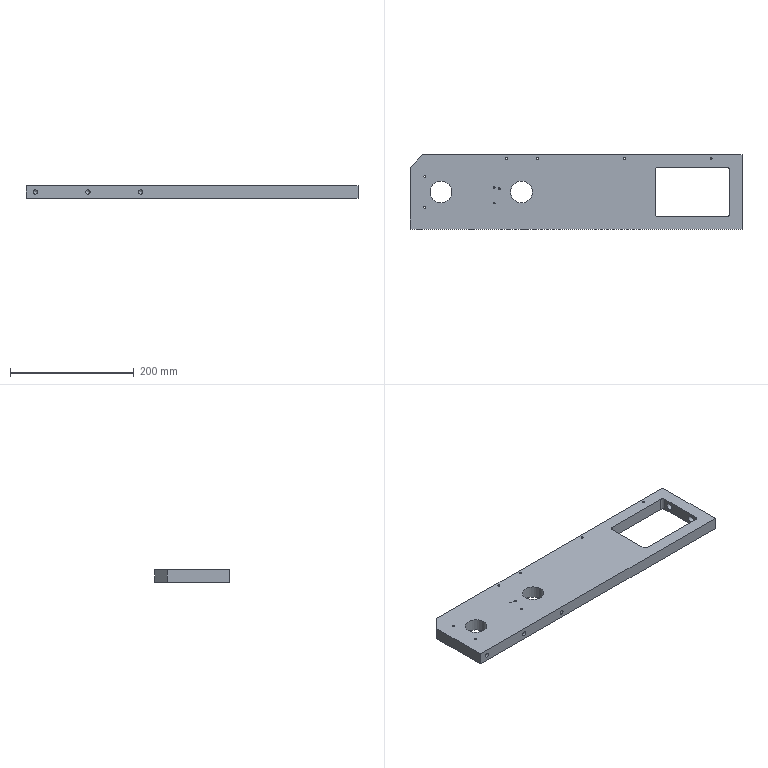Part | NX | 1 solid | 36 faces | box 536 x 120 x 20 mm | volume 1044762 mm3 | cylinder 20 | plane 11 | cone 5 | commonest cylinder face diameters 3.3 x7 10 x4 6.8 x3 2.5 x2 11 x2 35 x2
STEP:
#1=CARTESIAN_POINT('',(-248.,60.,10.));
#2=VERTEX_POINT('',#1);
#3=CARTESIAN_POINT('',(-268.,40.,10.));
#4=VERTEX_POINT('',#3);
#5=CARTESIAN_POINT('',(-268.,40.,10.));
#6=DIRECTION('',(-0.7071,-0.7071,0.));
#7=VECTOR('',#6,1000.);
#8=LINE('',#5,#7);
#9=EDGE_CURVE('',#2,#4,#8,.T.);
#10=ORIENTED_EDGE('',*,*,#9,.F.);
#11=CARTESIAN_POINT('',(-248.,60.,-10.));
#12=VERTEX_POINT('',#11);
#13=CARTESIAN_POINT('',(-248.,60.,10.));
#14=DIRECTION('',(0.,0.,1.));
#15=VECTOR('',#14,1000.);
#16=LINE('',#13,#15);
#17=EDGE_CURVE('',#12,#2,#16,.T.);
#18=ORIENTED_EDGE('',*,*,#17,.F.);
#19=CARTESIAN_POINT('',(-268.,40.,-10.));
#20=VERTEX_POINT('',#19);
#21=CARTESIAN_POINT('',(-154.,154.,-10.));
#22=DIRECTION('',(0.7071,0.7071,0.));
#23=VECTOR('',#22,1000.);
#24=LINE('',#21,#23);
#25=EDGE_CURVE('',#20,#12,#24,.T.);
#26=ORIENTED_EDGE('',*,*,#25,.F.);
#27=CARTESIAN_POINT('',(-268.,40.,10.));
#28=DIRECTION('',(0.,0.,-1.));
#29=VECTOR('',#28,1000.);
#30=LINE('',#27,#29);
#31=EDGE_CURVE('',#4,#20,#30,.T.);
#32=ORIENTED_EDGE('',*,*,#31,.F.);
#33=EDGE_LOOP('',(#10,#18,#26,#32));
#34=FACE_BOUND('',#33,.T.);
#35=CARTESIAN_POINT('',(-268.,40.,10.));
#36=DIRECTION('',(0.7071,-0.7071,0.));
#37=DIRECTION('',(0.,0.,-1.));
#38=AXIS2_PLACEMENT_3D('',#35,#36,#37);
#39=PLANE('',#38);
#40=ADVANCED_FACE('',(#34),#39,.F.);
#41=CARTESIAN_POINT('',(248.,-35.,10.));
#42=VERTEX_POINT('',#41);
#43=CARTESIAN_POINT('',(248.,35.,10.));
#44=VERTEX_POINT('',#43);
#45=CARTESIAN_POINT('',(248.,-35.,10.));
#46=DIRECTION('',(0.,1.,0.));
#47=VECTOR('',#46,1000.);
#48=LINE('',#45,#47);
#49=EDGE_CURVE('',#42,#44,#48,.T.);
#50=ORIENTED_EDGE('',*,*,#49,.T.);
#51=CARTESIAN_POINT('',(248.,35.,-10.));
#52=VERTEX_POINT('',#51);
#53=CARTESIAN_POINT('',(248.,35.,-10.));
#54=DIRECTION('',(0.,0.,1.));
#55=VECTOR('',#54,1000.);
#56=LINE('',#53,#55);
#57=EDGE_CURVE('',#52,#44,#56,.T.);
#58=ORIENTED_EDGE('',*,*,#57,.F.);
#59=CARTESIAN_POINT('',(248.,-35.,-10.));
#60=VERTEX_POINT('',#59);
#61=CARTESIAN_POINT('',(248.,-35.,-10.));
#62=DIRECTION('',(0.,1.,0.));
#63=VECTOR('',#62,1000.);
#64=LINE('',#61,#63);
#65=EDGE_CURVE('',#60,#52,#64,.T.);
#66=ORIENTED_EDGE('',*,*,#65,.F.);
#67=CARTESIAN_POINT('',(248.,-35.,-10.));
#68=DIRECTION('',(0.,0.,1.));
#69=VECTOR('',#68,1000.);
#70=LINE('',#67,#69);
#71=EDGE_CURVE('',#60,#42,#70,.T.);
#72=ORIENTED_EDGE('',*,*,#71,.T.);
#73=EDGE_LOOP('',(#50,#58,#66,#72));
#74=FACE_BOUND('',#73,.T.);
#75=CARTESIAN_POINT('',(248.,25.,-5.5));
#76=VERTEX_POINT('',#75);
#77=CARTESIAN_POINT('',(248.,25.,0.));
#78=DIRECTION('',(1.,0.,0.));
#79=DIRECTION('',(0.,0.,-1.));
#80=AXIS2_PLACEMENT_3D('',#77,#78,#79);
#81=CIRCLE('',#80,5.5);
#82=EDGE_CURVE('',#76,#76,#81,.T.);
#83=ORIENTED_EDGE('',*,*,#82,.T.);
#84=EDGE_LOOP('',(#83));
#85=FACE_BOUND('',#84,.T.);
#86=CARTESIAN_POINT('',(248.,-25.,-5.5));
#87=VERTEX_POINT('',#86);
#88=CARTESIAN_POINT('',(248.,-25.,0.));
#89=DIRECTION('',(1.,0.,0.));
#90=DIRECTION('',(0.,0.,-1.));
#91=AXIS2_PLACEMENT_3D('',#88,#89,#90);
#92=CIRCLE('',#91,5.5);
#93=EDGE_CURVE('',#87,#87,#92,.T.);
#94=ORIENTED_EDGE('',*,*,#93,.T.);
#95=EDGE_LOOP('',(#94));
#96=FACE_BOUND('',#95,.T.);
#97=CARTESIAN_POINT('',(248.,-35.,-10.));
#98=DIRECTION('',(1.,0.,0.));
#99=DIRECTION('',(0.,0.,-1.));
#100=AXIS2_PLACEMENT_3D('',#97,#98,#99);
#101=PLANE('',#100);
#102=ADVANCED_FACE('',(#74,#85,#96),#101,.F.);
#103=CARTESIAN_POINT('',(243.,40.,10.));
#104=VERTEX_POINT('',#103);
#105=CARTESIAN_POINT('',(243.,35.,10.));
#106=DIRECTION('',(0.,0.,1.));
#107=DIRECTION('',(-1.,0.,0.));
#108=AXIS2_PLACEMENT_3D('',#105,#106,#107);
#109=CIRCLE('',#108,5.);
#110=EDGE_CURVE('',#44,#104,#109,.T.);
#111=ORIENTED_EDGE('',*,*,#110,.T.);
#112=CARTESIAN_POINT('',(243.,40.,-10.));
#113=VERTEX_POINT('',#112);
#114=CARTESIAN_POINT('',(243.,40.,-10.));
#115=DIRECTION('',(0.,0.,1.));
#116=VECTOR('',#115,1000.);
#117=LINE('',#114,#116);
#118=EDGE_CURVE('',#113,#104,#117,.T.);
#119=ORIENTED_EDGE('',*,*,#118,.F.);
#120=CARTESIAN_POINT('',(243.,35.,-10.));
#121=DIRECTION('',(0.,0.,1.));
#122=DIRECTION('',(-1.,0.,0.));
#123=AXIS2_PLACEMENT_3D('',#120,#121,#122);
#124=CIRCLE('',#123,5.);
#125=EDGE_CURVE('',#52,#113,#124,.T.);
#126=ORIENTED_EDGE('',*,*,#125,.F.);
#127=ORIENTED_EDGE('',*,*,#57,.T.);
#128=EDGE_LOOP('',(#111,#119,#126,#127));
#129=FACE_BOUND('',#128,.T.);
#130=CARTESIAN_POINT('',(243.,35.,-10.));
#131=DIRECTION('',(0.,0.,1.));
#132=DIRECTION('',(1.,0.,0.));
#133=AXIS2_PLACEMENT_3D('',#130,#131,#132);
#134=CYLINDRICAL_SURFACE('',#133,5.);
#135=ADVANCED_FACE('',(#129),#134,.F.);
#136=CARTESIAN_POINT('',(133.,40.,10.));
#137=VERTEX_POINT('',#136);
#138=CARTESIAN_POINT('',(133.,40.,10.));
#139=DIRECTION('',(-1.,0.,0.));
#140=VECTOR('',#139,1000.);
#141=LINE('',#138,#140);
#142=EDGE_CURVE('',#104,#137,#141,.T.);
#143=ORIENTED_EDGE('',*,*,#142,.T.);
#144=CARTESIAN_POINT('',(133.,40.,-10.));
#145=VERTEX_POINT('',#144);
#146=CARTESIAN_POINT('',(133.,40.,-10.));
#147=DIRECTION('',(0.,0.,1.));
#148=VECTOR('',#147,1000.);
#149=LINE('',#146,#148);
#150=EDGE_CURVE('',#145,#137,#149,.T.);
#151=ORIENTED_EDGE('',*,*,#150,.F.);
#152=CARTESIAN_POINT('',(133.,40.,-10.));
#153=DIRECTION('',(-1.,0.,0.));
#154=VECTOR('',#153,1000.);
#155=LINE('',#152,#154);
#156=EDGE_CURVE('',#113,#145,#155,.T.);
#157=ORIENTED_EDGE('',*,*,#156,.F.);
#158=ORIENTED_EDGE('',*,*,#118,.T.);
#159=EDGE_LOOP('',(#143,#151,#157,#158));
#160=FACE_BOUND('',#159,.T.);
#161=CARTESIAN_POINT('',(133.,40.,-10.));
#162=DIRECTION('',(0.,1.,0.));
#163=DIRECTION('',(-1.,0.,0.));
#164=AXIS2_PLACEMENT_3D('',#161,#162,#163);
#165=PLANE('',#164);
#166=ADVANCED_FACE('',(#160),#165,.F.);
#167=CARTESIAN_POINT('',(128.,35.,10.));
#168=VERTEX_POINT('',#167);
#169=CARTESIAN_POINT('',(133.,35.,10.));
#170=DIRECTION('',(0.,0.,1.));
#171=DIRECTION('',(-1.,0.,0.));
#172=AXIS2_PLACEMENT_3D('',#169,#170,#171);
#173=CIRCLE('',#172,5.);
#174=EDGE_CURVE('',#137,#168,#173,.T.);
#175=ORIENTED_EDGE('',*,*,#174,.T.);
#176=CARTESIAN_POINT('',(128.,35.,-10.));
#177=VERTEX_POINT('',#176);
#178=CARTESIAN_POINT('',(128.,35.,-10.));
#179=DIRECTION('',(0.,0.,1.));
#180=VECTOR('',#179,1000.);
#181=LINE('',#178,#180);
#182=EDGE_CURVE('',#177,#168,#181,.T.);
#183=ORIENTED_EDGE('',*,*,#182,.F.);
#184=CARTESIAN_POINT('',(133.,35.,-10.));
#185=DIRECTION('',(0.,0.,1.));
#186=DIRECTION('',(-1.,0.,0.));
#187=AXIS2_PLACEMENT_3D('',#184,#185,#186);
#188=CIRCLE('',#187,5.);
#189=EDGE_CURVE('',#145,#177,#188,.T.);
#190=ORIENTED_EDGE('',*,*,#189,.F.);
#191=ORIENTED_EDGE('',*,*,#150,.T.);
#192=EDGE_LOOP('',(#175,#183,#190,#191));
#193=FACE_BOUND('',#192,.T.);
#194=CARTESIAN_POINT('',(133.,35.,-10.));
#195=DIRECTION('',(0.,0.,1.));
#196=DIRECTION('',(1.,0.,0.));
#197=AXIS2_PLACEMENT_3D('',#194,#195,#196);
#198=CYLINDRICAL_SURFACE('',#197,5.);
#199=ADVANCED_FACE('',(#193),#198,.F.);
#200=CARTESIAN_POINT('',(128.,-35.,10.));
#201=VERTEX_POINT('',#200);
#202=CARTESIAN_POINT('',(128.,-35.,10.));
#203=DIRECTION('',(0.,-1.,0.));
#204=VECTOR('',#203,1000.);
#205=LINE('',#202,#204);
#206=EDGE_CURVE('',#168,#201,#205,.T.);
#207=ORIENTED_EDGE('',*,*,#206,.T.);
#208=CARTESIAN_POINT('',(128.,-35.,-10.));
#209=VERTEX_POINT('',#208);
#210=CARTESIAN_POINT('',(128.,-35.,-10.));
#211=DIRECTION('',(0.,0.,1.));
#212=VECTOR('',#211,1000.);
#213=LINE('',#210,#212);
#214=EDGE_CURVE('',#209,#201,#213,.T.);
#215=ORIENTED_EDGE('',*,*,#214,.F.);
#216=CARTESIAN_POINT('',(128.,-35.,-10.));
#217=DIRECTION('',(0.,-1.,0.));
#218=VECTOR('',#217,1000.);
#219=LINE('',#216,#218);
#220=EDGE_CURVE('',#177,#209,#219,.T.);
#221=ORIENTED_EDGE('',*,*,#220,.F.);
#222=ORIENTED_EDGE('',*,*,#182,.T.);
#223=EDGE_LOOP('',(#207,#215,#221,#222));
#224=FACE_BOUND('',#223,.T.);
#225=CARTESIAN_POINT('',(128.,-35.,-10.));
#226=DIRECTION('',(-1.,0.,0.));
#227=DIRECTION('',(0.,0.,1.));
#228=AXIS2_PLACEMENT_3D('',#225,#226,#227);
#229=PLANE('',#228);
#230=ADVANCED_FACE('',(#224),#229,.F.);
#231=CARTESIAN_POINT('',(133.,-40.,10.));
#232=VERTEX_POINT('',#231);
#233=CARTESIAN_POINT('',(133.,-35.,10.));
#234=DIRECTION('',(0.,0.,1.));
#235=DIRECTION('',(-1.,0.,0.));
#236=AXIS2_PLACEMENT_3D('',#233,#234,#235);
#237=CIRCLE('',#236,5.);
#238=EDGE_CURVE('',#201,#232,#237,.T.);
#239=ORIENTED_EDGE('',*,*,#238,.T.);
#240=CARTESIAN_POINT('',(133.,-40.,-10.));
#241=VERTEX_POINT('',#240);
#242=CARTESIAN_POINT('',(133.,-40.,-10.));
#243=DIRECTION('',(0.,0.,1.));
#244=VECTOR('',#243,1000.);
#245=LINE('',#242,#244);
#246=EDGE_CURVE('',#241,#232,#245,.T.);
#247=ORIENTED_EDGE('',*,*,#246,.F.);
#248=CARTESIAN_POINT('',(133.,-35.,-10.));
#249=DIRECTION('',(0.,0.,1.));
#250=DIRECTION('',(-1.,0.,0.));
#251=AXIS2_PLACEMENT_3D('',#248,#249,#250);
#252=CIRCLE('',#251,5.);
#253=EDGE_CURVE('',#209,#241,#252,.T.);
#254=ORIENTED_EDGE('',*,*,#253,.F.);
#255=ORIENTED_EDGE('',*,*,#214,.T.);
#256=EDGE_LOOP('',(#239,#247,#254,#255));
#257=FACE_BOUND('',#256,.T.);
#258=CARTESIAN_POINT('',(133.,-35.,-10.));
#259=DIRECTION('',(0.,0.,1.));
#260=DIRECTION('',(1.,0.,0.));
#261=AXIS2_PLACEMENT_3D('',#258,#259,#260);
#262=CYLINDRICAL_SURFACE('',#261,5.);
#263=ADVANCED_FACE('',(#257),#262,.F.);
#264=CARTESIAN_POINT('',(243.,-40.,10.));
#265=VERTEX_POINT('',#264);
#266=CARTESIAN_POINT('',(133.,-40.,10.));
#267=DIRECTION('',(1.,0.,0.));
#268=VECTOR('',#267,1000.);
#269=LINE('',#266,#268);
#270=EDGE_CURVE('',#232,#265,#269,.T.);
#271=ORIENTED_EDGE('',*,*,#270,.T.);
#272=CARTESIAN_POINT('',(243.,-40.,-10.));
#273=VERTEX_POINT('',#272);
#274=CARTESIAN_POINT('',(243.,-40.,-10.));
#275=DIRECTION('',(0.,0.,1.));
#276=VECTOR('',#275,1000.);
#277=LINE('',#274,#276);
#278=EDGE_CURVE('',#273,#265,#277,.T.);
#279=ORIENTED_EDGE('',*,*,#278,.F.);
#280=CARTESIAN_POINT('',(133.,-40.,-10.));
#281=DIRECTION('',(1.,0.,0.));
#282=VECTOR('',#281,1000.);
#283=LINE('',#280,#282);
#284=EDGE_CURVE('',#241,#273,#283,.T.);
#285=ORIENTED_EDGE('',*,*,#284,.F.);
#286=ORIENTED_EDGE('',*,*,#246,.T.);
#287=EDGE_LOOP('',(#271,#279,#285,#286));
#288=FACE_BOUND('',#287,.T.);
#289=CARTESIAN_POINT('',(133.,-40.,-10.));
#290=DIRECTION('',(0.,-1.,0.));
#291=DIRECTION('',(0.,0.,-1.));
#292=AXIS2_PLACEMENT_3D('',#289,#290,#291);
#293=PLANE('',#292);
#294=ADVANCED_FACE('',(#288),#293,.F.);
#295=CARTESIAN_POINT('',(243.,-35.,10.));
#296=DIRECTION('',(0.,0.,1.));
#297=DIRECTION('',(1.,0.,0.));
#298=AXIS2_PLACEMENT_3D('',#295,#296,#297);
#299=CIRCLE('',#298,5.);
#300=EDGE_CURVE('',#265,#42,#299,.T.);
#301=ORIENTED_EDGE('',*,*,#300,.T.);
#302=ORIENTED_EDGE('',*,*,#71,.F.);
#303=CARTESIAN_POINT('',(243.,-35.,-10.));
#304=DIRECTION('',(0.,0.,1.));
#305=DIRECTION('',(1.,0.,0.));
#306=AXIS2_PLACEMENT_3D('',#303,#304,#305);
#307=CIRCLE('',#306,5.);
#308=EDGE_CURVE('',#273,#60,#307,.T.);
#309=ORIENTED_EDGE('',*,*,#308,.F.);
#310=ORIENTED_EDGE('',*,*,#278,.T.);
#311=EDGE_LOOP('',(#301,#302,#309,#310));
#312=FACE_BOUND('',#311,.T.);
#313=CARTESIAN_POINT('',(243.,-35.,-10.));
#314=DIRECTION('',(0.,0.,1.));
#315=DIRECTION('',(1.,0.,0.));
#316=AXIS2_PLACEMENT_3D('',#313,#314,#315);
#317=CYLINDRICAL_SURFACE('',#316,5.);
#318=ADVANCED_FACE('',(#312),#317,.F.);
#319=ORIENTED_EDGE('',*,*,#308,.T.);
#320=ORIENTED_EDGE('',*,*,#65,.T.);
#321=ORIENTED_EDGE('',*,*,#125,.T.);
#322=ORIENTED_EDGE('',*,*,#156,.T.);
#323=ORIENTED_EDGE('',*,*,#189,.T.);
#324=ORIENTED_EDGE('',*,*,#220,.T.);
#325=ORIENTED_EDGE('',*,*,#253,.T.);
#326=ORIENTED_EDGE('',*,*,#284,.T.);
#327=EDGE_LOOP('',(#319,#320,#321,#322,#323,#324,#325,#326));
#328=FACE_BOUND('',#327,.T.);
#329=CARTESIAN_POINT('',(-268.,-60.,-10.));
#330=VERTEX_POINT('',#329);
#331=CARTESIAN_POINT('',(-268.,-60.,-10.));
#332=DIRECTION('',(0.,-1.,0.));
#333=VECTOR('',#332,1000.);
#334=LINE('',#331,#333);
#335=EDGE_CURVE('',#20,#330,#334,.T.);
#336=ORIENTED_EDGE('',*,*,#335,.F.);
#337=ORIENTED_EDGE('',*,*,#25,.T.);
#338=CARTESIAN_POINT('',(268.,60.,-10.));
#339=VERTEX_POINT('',#338);
#340=CARTESIAN_POINT('',(-268.,60.,-10.));
#341=DIRECTION('',(-1.,0.,0.));
#342=VECTOR('',#341,1000.);
#343=LINE('',#340,#342);
#344=EDGE_CURVE('',#339,#12,#343,.T.);
#345=ORIENTED_EDGE('',*,*,#344,.F.);
#346=CARTESIAN_POINT('',(268.,-60.,-10.));
#347=VERTEX_POINT('',#346);
#348=CARTESIAN_POINT('',(268.,-60.,-10.));
#349=DIRECTION('',(0.,1.,0.));
#350=VECTOR('',#349,1000.);
#351=LINE('',#348,#350);
#352=EDGE_CURVE('',#339,#347,#351,.F.);
#353=ORIENTED_EDGE('',*,*,#352,.T.);
#354=CARTESIAN_POINT('',(-268.,-60.,-10.));
#355=DIRECTION('',(1.,0.,0.));
#356=VECTOR('',#355,1000.);
#357=LINE('',#354,#356);
#358=EDGE_CURVE('',#330,#347,#357,.T.);
#359=ORIENTED_EDGE('',*,*,#358,.F.);
#360=EDGE_LOOP('',(#336,#337,#345,#353,#359));
#361=FACE_BOUND('',#360,.T.);
#362=CARTESIAN_POINT('',(-245.65,25.,-10.));
#363=VERTEX_POINT('',#362);
#364=CARTESIAN_POINT('',(-244.,25.,-10.));
#365=DIRECTION('',(0.,0.,-1.));
#366=DIRECTION('',(-1.,0.,0.));
#367=AXIS2_PLACEMENT_3D('',#364,#365,#366);
#368=CIRCLE('',#367,1.65);
#369=EDGE_CURVE('',#363,#363,#368,.T.);
#370=ORIENTED_EDGE('',*,*,#369,.F.);
#371=EDGE_LOOP('',(#370));
#372=FACE_BOUND('',#371,.T.);
#373=CARTESIAN_POINT('',(-245.65,-25.,-10.));
#374=VERTEX_POINT('',#373);
#375=CARTESIAN_POINT('',(-244.,-25.,-10.));
#376=DIRECTION('',(0.,0.,-1.));
#377=DIRECTION('',(-1.,0.,0.));
#378=AXIS2_PLACEMENT_3D('',#375,#376,#377);
#379=CIRCLE('',#378,1.65);
#380=EDGE_CURVE('',#374,#374,#379,.T.);
#381=ORIENTED_EDGE('',*,*,#380,.F.);
#382=EDGE_LOOP('',(#381));
#383=FACE_BOUND('',#382,.T.);
#384=CARTESIAN_POINT('',(-70.5,0.,-10.));
#385=VERTEX_POINT('',#384);
#386=CARTESIAN_POINT('',(-88.,0.,-10.));
#387=DIRECTION('',(0.,0.,1.));
#388=DIRECTION('',(1.,0.,0.));
#389=AXIS2_PLACEMENT_3D('',#386,#387,#388);
#390=CIRCLE('',#389,17.5);
#391=EDGE_CURVE('',#385,#385,#390,.T.);
#392=ORIENTED_EDGE('',*,*,#391,.T.);
#393=EDGE_LOOP('',(#392));
#394=FACE_BOUND('',#393,.T.);
#395=CARTESIAN_POINT('',(-200.5,0.,-10.));
#396=VERTEX_POINT('',#395);
#397=CARTESIAN_POINT('',(-218.,0.,-10.));
#398=DIRECTION('',(0.,0.,1.));
#399=DIRECTION('',(1.,0.,0.));
#400=AXIS2_PLACEMENT_3D('',#397,#398,#399);
#401=CIRCLE('',#400,17.5);
#402=EDGE_CURVE('',#396,#396,#401,.T.);
#403=ORIENTED_EDGE('',*,*,#402,.T.);
#404=EDGE_LOOP('',(#403));
#405=FACE_BOUND('',#404,.T.);
#406=CARTESIAN_POINT('',(219.65,54.25,-10.));
#407=VERTEX_POINT('',#406);
#408=CARTESIAN_POINT('',(218.,54.25,-10.));
#409=DIRECTION('',(0.,0.,1.));
#410=DIRECTION('',(1.,0.,0.));
#411=AXIS2_PLACEMENT_3D('',#408,#409,#410);
#412=CIRCLE('',#411,1.65);
#413=EDGE_CURVE('',#407,#407,#412,.T.);
#414=ORIENTED_EDGE('',*,*,#413,.T.);
#415=EDGE_LOOP('',(#414));
#416=FACE_BOUND('',#415,.T.);
#417=CARTESIAN_POINT('',(79.65,54.25,-10.));
#418=VERTEX_POINT('',#417);
#419=CARTESIAN_POINT('',(78.,54.25,-10.));
#420=DIRECTION('',(0.,0.,1.));
#421=DIRECTION('',(1.,0.,0.));
#422=AXIS2_PLACEMENT_3D('',#419,#420,#421);
#423=CIRCLE('',#422,1.65);
#424=EDGE_CURVE('',#418,#418,#423,.T.);
#425=ORIENTED_EDGE('',*,*,#424,.T.);
#426=EDGE_LOOP('',(#425));
#427=FACE_BOUND('',#426,.T.);
#428=CARTESIAN_POINT('',(-60.35,54.25,-10.));
#429=VERTEX_POINT('',#428);
#430=CARTESIAN_POINT('',(-62.,54.25,-10.));
#431=DIRECTION('',(0.,0.,1.));
#432=DIRECTION('',(1.,0.,0.));
#433=AXIS2_PLACEMENT_3D('',#430,#431,#432);
#434=CIRCLE('',#433,1.65);
#435=EDGE_CURVE('',#429,#429,#434,.T.);
#436=ORIENTED_EDGE('',*,*,#435,.T.);
#437=EDGE_LOOP('',(#436));
#438=FACE_BOUND('',#437,.T.);
#439=CARTESIAN_POINT('',(-110.35,54.25,-10.));
#440=VERTEX_POINT('',#439);
#441=CARTESIAN_POINT('',(-112.,54.25,-10.));
#442=DIRECTION('',(0.,0.,1.));
#443=DIRECTION('',(1.,0.,0.));
#444=AXIS2_PLACEMENT_3D('',#441,#442,#443);
#445=CIRCLE('',#444,1.65);
#446=EDGE_CURVE('',#440,#440,#445,.T.);
#447=ORIENTED_EDGE('',*,*,#446,.T.);
#448=EDGE_LOOP('',(#447));
#449=FACE_BOUND('',#448,.T.);
#450=CARTESIAN_POINT('',(-122.35,5.25,-10.));
#451=VERTEX_POINT('',#450);
#452=CARTESIAN_POINT('',(-124.,5.25,-10.));
#453=DIRECTION('',(0.,0.,1.));
#454=DIRECTION('',(1.,0.,0.));
#455=AXIS2_PLACEMENT_3D('',#452,#453,#454);
#456=CIRCLE('',#455,1.65);
#457=EDGE_CURVE('',#451,#451,#456,.T.);
#458=ORIENTED_EDGE('',*,*,#457,.T.);
#459=EDGE_LOOP('',(#458));
#460=FACE_BOUND('',#459,.T.);
#461=CARTESIAN_POINT('',(0.,0.,-10.));
#462=DIRECTION('',(0.,0.,-1.));
#463=DIRECTION('',(-1.,0.,0.));
#464=AXIS2_PLACEMENT_3D('',#461,#462,#463);
#465=PLANE('',#464);
#466=ADVANCED_FACE('',(#328,#361,#372,#383,#394,#405,#416,#427,#438,#449,#460),#465,.T.);
#467=CARTESIAN_POINT('',(268.,60.,10.));
#468=VERTEX_POINT('',#467);
#469=CARTESIAN_POINT('',(-268.,60.,10.));
#470=DIRECTION('',(-1.,0.,0.));
#471=VECTOR('',#470,1000.);
#472=LINE('',#469,#471);
#473=EDGE_CURVE('',#468,#2,#472,.T.);
#474=ORIENTED_EDGE('',*,*,#473,.T.);
#475=ORIENTED_EDGE('',*,*,#9,.T.);
#476=CARTESIAN_POINT('',(-268.,-60.,10.));
#477=VERTEX_POINT('',#476);
#478=CARTESIAN_POINT('',(-268.,-60.,10.));
#479=DIRECTION('',(0.,-1.,0.));
#480=VECTOR('',#479,1000.);
#481=LINE('',#478,#480);
#482=EDGE_CURVE('',#4,#477,#481,.T.);
#483=ORIENTED_EDGE('',*,*,#482,.T.);
#484=CARTESIAN_POINT('',(268.,-60.,10.));
#485=VERTEX_POINT('',#484);
#486=CARTESIAN_POINT('',(-268.,-60.,10.));
#487=DIRECTION('',(1.,0.,0.));
#488=VECTOR('',#487,1000.);
#489=LINE('',#486,#488);
#490=EDGE_CURVE('',#485,#477,#489,.F.);
#491=ORIENTED_EDGE('',*,*,#490,.F.);
#492=CARTESIAN_POINT('',(268.,-60.,10.));
#493=DIRECTION('',(0.,1.,0.));
#494=VECTOR('',#493,1000.);
#495=LINE('',#492,#494);
#496=EDGE_CURVE('',#468,#485,#495,.F.);
#497=ORIENTED_EDGE('',*,*,#496,.F.);
#498=EDGE_LOOP('',(#474,#475,#483,#491,#497));
#499=FACE_BOUND('',#498,.T.);
#500=ORIENTED_EDGE('',*,*,#49,.F.);
#501=ORIENTED_EDGE('',*,*,#300,.F.);
#502=ORIENTED_EDGE('',*,*,#270,.F.);
#503=ORIENTED_EDGE('',*,*,#238,.F.);
#504=ORIENTED_EDGE('',*,*,#206,.F.);
#505=ORIENTED_EDGE('',*,*,#174,.F.);
#506=ORIENTED_EDGE('',*,*,#142,.F.);
#507=ORIENTED_EDGE('',*,*,#110,.F.);
#508=EDGE_LOOP('',(#500,#501,#502,#503,#504,#505,#506,#507));
#509=FACE_BOUND('',#508,.T.);
#510=CARTESIAN_POINT('',(-245.65,25.,10.));
#511=VERTEX_POINT('',#510);
#512=CARTESIAN_POINT('',(-244.,25.,10.));
#513=DIRECTION('',(0.,0.,-1.));
#514=DIRECTION('',(-1.,0.,0.));
#515=AXIS2_PLACEMENT_3D('',#512,#513,#514);
#516=CIRCLE('',#515,1.65);
#517=EDGE_CURVE('',#511,#511,#516,.T.);
#518=ORIENTED_EDGE('',*,*,#517,.T.);
#519=EDGE_LOOP('',(#518));
#520=FACE_BOUND('',#519,.T.);
#521=CARTESIAN_POINT('',(-245.65,-25.,10.));
#522=VERTEX_POINT('',#521);
#523=CARTESIAN_POINT('',(-244.,-25.,10.));
#524=DIRECTION('',(0.,0.,-1.));
#525=DIRECTION('',(-1.,0.,0.));
#526=AXIS2_PLACEMENT_3D('',#523,#524,#525);
#527=CIRCLE('',#526,1.65);
#528=EDGE_CURVE('',#522,#522,#527,.T.);
#529=ORIENTED_EDGE('',*,*,#528,.T.);
#530=EDGE_LOOP('',(#529));
#531=FACE_BOUND('',#530,.T.);
#532=CARTESIAN_POINT('',(-70.5,0.,10.));
#533=VERTEX_POINT('',#532);
#534=CARTESIAN_POINT('',(-88.,0.,10.));
#535=DIRECTION('',(0.,0.,1.));
#536=DIRECTION('',(1.,0.,0.));
#537=AXIS2_PLACEMENT_3D('',#534,#535,#536);
#538=CIRCLE('',#537,17.5);
#539=EDGE_CURVE('',#533,#533,#538,.T.);
#540=ORIENTED_EDGE('',*,*,#539,.F.);
#541=EDGE_LOOP('',(#540));
#542=FACE_BOUND('',#541,.T.);
#543=CARTESIAN_POINT('',(-200.5,0.,10.));
#544=VERTEX_POINT('',#543);
#545=CARTESIAN_POINT('',(-218.,0.,10.));
#546=DIRECTION('',(0.,0.,1.));
#547=DIRECTION('',(1.,0.,0.));
#548=AXIS2_PLACEMENT_3D('',#545,#546,#547);
#549=CIRCLE('',#548,17.5);
#550=EDGE_CURVE('',#544,#544,#549,.T.);
#551=ORIENTED_EDGE('',*,*,#550,.F.);
#552=EDGE_LOOP('',(#551));
#553=FACE_BOUND('',#552,.T.);
#554=CARTESIAN_POINT('',(-130.75,-18.,10.));
#555=VERTEX_POINT('',#554);
#556=CARTESIAN_POINT('',(-132.,-18.,10.));
#557=DIRECTION('',(0.,0.,1.));
#558=DIRECTION('',(1.,0.,0.));
#559=AXIS2_PLACEMENT_3D('',#556,#557,#558);
#560=CIRCLE('',#559,1.25);
#561=EDGE_CURVE('',#555,#555,#560,.T.);
#562=ORIENTED_EDGE('',*,*,#561,.F.);
#563=EDGE_LOOP('',(#562));
#564=FACE_BOUND('',#563,.T.);
#565=CARTESIAN_POINT('',(-130.75,7.,10.));
#566=VERTEX_POINT('',#565);
#567=CARTESIAN_POINT('',(-132.,7.,10.));
#568=DIRECTION('',(0.,0.,1.));
#569=DIRECTION('',(1.,0.,0.));
#570=AXIS2_PLACEMENT_3D('',#567,#568,#569);
#571=CIRCLE('',#570,1.25);
#572=EDGE_CURVE('',#566,#566,#571,.T.);
#573=ORIENTED_EDGE('',*,*,#572,.F.);
#574=EDGE_LOOP('',(#573));
#575=FACE_BOUND('',#574,.T.);
#576=CARTESIAN_POINT('',(219.65,54.25,10.));
#577=VERTEX_POINT('',#576);
#578=CARTESIAN_POINT('',(218.,54.25,10.));
#579=DIRECTION('',(0.,0.,1.));
#580=DIRECTION('',(1.,0.,0.));
#581=AXIS2_PLACEMENT_3D('',#578,#579,#580);
#582=CIRCLE('',#581,1.65);
#583=EDGE_CURVE('',#577,#577,#582,.T.);
#584=ORIENTED_EDGE('',*,*,#583,.F.);
#585=EDGE_LOOP('',(#584));
#586=FACE_BOUND('',#585,.T.);
#587=CARTESIAN_POINT('',(79.65,54.25,10.));
#588=VERTEX_POINT('',#587);
#589=CARTESIAN_POINT('',(78.,54.25,10.));
#590=DIRECTION('',(0.,0.,1.));
#591=DIRECTION('',(1.,0.,0.));
#592=AXIS2_PLACEMENT_3D('',#589,#590,#591);
#593=CIRCLE('',#592,1.65);
#594=EDGE_CURVE('',#588,#588,#593,.T.);
#595=ORIENTED_EDGE('',*,*,#594,.F.);
#596=EDGE_LOOP('',(#595));
#597=FACE_BOUND('',#596,.T.);
#598=CARTESIAN_POINT('',(-60.35,54.25,10.));
#599=VERTEX_POINT('',#598);
#600=CARTESIAN_POINT('',(-62.,54.25,10.));
#601=DIRECTION('',(0.,0.,1.));
#602=DIRECTION('',(1.,0.,0.));
#603=AXIS2_PLACEMENT_3D('',#600,#601,#602);
#604=CIRCLE('',#603,1.65);
#605=EDGE_CURVE('',#599,#599,#604,.T.);
#606=ORIENTED_EDGE('',*,*,#605,.F.);
#607=EDGE_LOOP('',(#606));
#608=FACE_BOUND('',#607,.T.);
#609=CARTESIAN_POINT('',(-110.35,54.25,10.));
#610=VERTEX_POINT('',#609);
#611=CARTESIAN_POINT('',(-112.,54.25,10.));
#612=DIRECTION('',(0.,0.,1.));
#613=DIRECTION('',(1.,0.,0.));
#614=AXIS2_PLACEMENT_3D('',#611,#612,#613);
#615=CIRCLE('',#614,1.65);
#616=EDGE_CURVE('',#610,#610,#615,.T.);
#617=ORIENTED_EDGE('',*,*,#616,.F.);
#618=EDGE_LOOP('',(#617));
#619=FACE_BOUND('',#618,.T.);
#620=CARTESIAN_POINT('',(-122.35,5.25,10.));
#621=VERTEX_POINT('',#620);
#622=CARTESIAN_POINT('',(-124.,5.25,10.));
#623=DIRECTION('',(0.,0.,1.));
#624=DIRECTION('',(1.,0.,0.));
#625=AXIS2_PLACEMENT_3D('',#622,#623,#624);
#626=CIRCLE('',#625,1.65);
#627=EDGE_CURVE('',#621,#621,#626,.T.);
#628=ORIENTED_EDGE('',*,*,#627,.F.);
#629=EDGE_LOOP('',(#628));
#630=FACE_BOUND('',#629,.T.);
#631=CARTESIAN_POINT('',(0.,0.,10.));
#632=DIRECTION('',(0.,0.,-1.));
#633=DIRECTION('',(-1.,0.,0.));
#634=AXIS2_PLACEMENT_3D('',#631,#632,#633);
#635=PLANE('',#634);
#636=ADVANCED_FACE('',(#499,#509,#520,#531,#542,#553,#564,#575,#586,#597,#608,#619,#630),#635,.F.);
#637=ORIENTED_EDGE('',*,*,#344,.T.);
#638=ORIENTED_EDGE('',*,*,#17,.T.);
#639=ORIENTED_EDGE('',*,*,#473,.F.);
#640=CARTESIAN_POINT('',(268.,60.,10.));
#641=DIRECTION('',(0.,0.,-1.));
#642=VECTOR('',#641,1000.);
#643=LINE('',#640,#642);
#644=EDGE_CURVE('',#468,#339,#643,.T.);
#645=ORIENTED_EDGE('',*,*,#644,.T.);
#646=EDGE_LOOP('',(#637,#638,#639,#645));
#647=FACE_BOUND('',#646,.T.);
#648=CARTESIAN_POINT('',(-268.,60.,10.));
#649=DIRECTION('',(0.,-1.,0.));
#650=DIRECTION('',(0.,0.,-1.));
#651=AXIS2_PLACEMENT_3D('',#648,#649,#650);
#652=PLANE('',#651);
#653=ADVANCED_FACE('',(#647),#652,.F.);
#654=ORIENTED_EDGE('',*,*,#482,.F.);
#655=ORIENTED_EDGE('',*,*,#31,.T.);
#656=ORIENTED_EDGE('',*,*,#335,.T.);
#657=CARTESIAN_POINT('',(-268.,-60.,10.));
#658=DIRECTION('',(0.,0.,-1.));
#659=VECTOR('',#658,1000.);
#660=LINE('',#657,#659);
#661=EDGE_CURVE('',#477,#330,#660,.T.);
#662=ORIENTED_EDGE('',*,*,#661,.F.);
#663=EDGE_LOOP('',(#654,#655,#656,#662));
#664=FACE_BOUND('',#663,.T.);
#665=CARTESIAN_POINT('',(-268.,-60.,10.));
#666=DIRECTION('',(1.,0.,0.));
#667=DIRECTION('',(0.,0.,-1.));
#668=AXIS2_PLACEMENT_3D('',#665,#666,#667);
#669=PLANE('',#668);
#670=ADVANCED_FACE('',(#664),#669,.F.);
#671=ORIENTED_EDGE('',*,*,#490,.T.);
#672=ORIENTED_EDGE('',*,*,#661,.T.);
#673=ORIENTED_EDGE('',*,*,#358,.T.);
#674=CARTESIAN_POINT('',(268.,-60.,10.));
#675=DIRECTION('',(0.,0.,-1.));
#676=VECTOR('',#675,1000.);
#677=LINE('',#674,#676);
#678=EDGE_CURVE('',#485,#347,#677,.T.);
#679=ORIENTED_EDGE('',*,*,#678,.F.);
#680=EDGE_LOOP('',(#671,#672,#673,#679));
#681=FACE_BOUND('',#680,.T.);
#682=CARTESIAN_POINT('',(-168.,-60.,-3.4));
#683=VERTEX_POINT('',#682);
#684=CARTESIAN_POINT('',(-168.,-60.,0.));
#685=DIRECTION('',(0.,-1.,0.));
#686=DIRECTION('',(0.,0.,-1.));
#687=AXIS2_PLACEMENT_3D('',#684,#685,#686);
#688=CIRCLE('',#687,3.4);
#689=EDGE_CURVE('',#683,#683,#688,.T.);
#690=ORIENTED_EDGE('',*,*,#689,.F.);
#691=EDGE_LOOP('',(#690));
#692=FACE_BOUND('',#691,.T.);
#693=CARTESIAN_POINT('',(-83.,-60.,-3.4));
#694=VERTEX_POINT('',#693);
#695=CARTESIAN_POINT('',(-83.,-60.,0.));
#696=DIRECTION('',(0.,-1.,0.));
#697=DIRECTION('',(0.,0.,-1.));
#698=AXIS2_PLACEMENT_3D('',#695,#696,#697);
#699=CIRCLE('',#698,3.4);
#700=EDGE_CURVE('',#694,#694,#699,.T.);
#701=ORIENTED_EDGE('',*,*,#700,.F.);
#702=EDGE_LOOP('',(#701));
#703=FACE_BOUND('',#702,.T.);
#704=CARTESIAN_POINT('',(-253.,-60.,-3.4));
#705=VERTEX_POINT('',#704);
#706=CARTESIAN_POINT('',(-253.,-60.,0.));
#707=DIRECTION('',(0.,-1.,0.));
#708=DIRECTION('',(0.,0.,-1.));
#709=AXIS2_PLACEMENT_3D('',#706,#707,#708);
#710=CIRCLE('',#709,3.4);
#711=EDGE_CURVE('',#705,#705,#710,.T.);
#712=ORIENTED_EDGE('',*,*,#711,.F.);
#713=EDGE_LOOP('',(#712));
#714=FACE_BOUND('',#713,.T.);
#715=CARTESIAN_POINT('',(-268.,-60.,10.));
#716=DIRECTION('',(0.,1.,0.));
#717=DIRECTION('',(0.,0.,1.));
#718=AXIS2_PLACEMENT_3D('',#715,#716,#717);
#719=PLANE('',#718);
#720=ADVANCED_FACE('',(#681,#692,#703,#714),#719,.F.);
#721=ORIENTED_EDGE('',*,*,#352,.F.);
#722=ORIENTED_EDGE('',*,*,#644,.F.);
#723=ORIENTED_EDGE('',*,*,#496,.T.);
#724=ORIENTED_EDGE('',*,*,#678,.T.);
#725=EDGE_LOOP('',(#721,#722,#723,#724));
#726=FACE_BOUND('',#725,.T.);
#727=CARTESIAN_POINT('',(268.,-25.,-5.5));
#728=VERTEX_POINT('',#727);
#729=CARTESIAN_POINT('',(268.,-25.,0.));
#730=DIRECTION('',(1.,0.,0.));
#731=DIRECTION('',(0.,0.,-1.));
#732=AXIS2_PLACEMENT_3D('',#729,#730,#731);
#733=CIRCLE('',#732,5.5);
#734=EDGE_CURVE('',#728,#728,#733,.T.);
#735=ORIENTED_EDGE('',*,*,#734,.F.);
#736=EDGE_LOOP('',(#735));
#737=FACE_BOUND('',#736,.T.);
#738=CARTESIAN_POINT('',(268.,25.,-5.5));
#739=VERTEX_POINT('',#738);
#740=CARTESIAN_POINT('',(268.,25.,0.));
#741=DIRECTION('',(1.,0.,0.));
#742=DIRECTION('',(0.,0.,-1.));
#743=AXIS2_PLACEMENT_3D('',#740,#741,#742);
#744=CIRCLE('',#743,5.5);
#745=EDGE_CURVE('',#739,#739,#744,.T.);
#746=ORIENTED_EDGE('',*,*,#745,.F.);
#747=EDGE_LOOP('',(#746));
#748=FACE_BOUND('',#747,.T.);
#749=CARTESIAN_POINT('',(268.,-60.,10.));
#750=DIRECTION('',(-1.,0.,0.));
#751=DIRECTION('',(0.,0.,1.));
#752=AXIS2_PLACEMENT_3D('',#749,#750,#751);
#753=PLANE('',#752);
#754=ADVANCED_FACE('',(#726,#737,#748),#753,.F.);
#755=CARTESIAN_POINT('',(-83.,-35.707,0.));
#756=VERTEX_POINT('',#755);
#757=VERTEX_LOOP('',#756);
#758=FACE_BOUND('',#757,.T.);
#759=CARTESIAN_POINT('',(-83.,-37.75,-3.4));
#760=VERTEX_POINT('',#759);
#761=CARTESIAN_POINT('',(-83.,-37.75,0.));
#762=DIRECTION('',(0.,-1.,0.));
#763=DIRECTION('',(0.,0.,-1.));
#764=AXIS2_PLACEMENT_3D('',#761,#762,#763);
#765=CIRCLE('',#764,3.4);
#766=EDGE_CURVE('',#760,#760,#765,.T.);
#767=ORIENTED_EDGE('',*,*,#766,.T.);
#768=EDGE_LOOP('',(#767));
#769=FACE_BOUND('',#768,.T.);
#770=CARTESIAN_POINT('',(-83.,-37.75,0.));
#771=DIRECTION('',(0.,-1.,0.));
#772=DIRECTION('',(0.,0.,-1.));
#773=AXIS2_PLACEMENT_3D('',#770,#771,#772);
#774=CONICAL_SURFACE('',#773,3.4,1.03);
#775=ADVANCED_FACE('',(#758,#769),#774,.F.);
#776=ORIENTED_EDGE('',*,*,#700,.T.);
#777=EDGE_LOOP('',(#776));
#778=FACE_BOUND('',#777,.T.);
#779=ORIENTED_EDGE('',*,*,#766,.F.);
#780=EDGE_LOOP('',(#779));
#781=FACE_BOUND('',#780,.T.);
#782=CARTESIAN_POINT('',(-83.,-60.,0.));
#783=DIRECTION('',(0.,-1.,0.));
#784=DIRECTION('',(0.,0.,-1.));
#785=AXIS2_PLACEMENT_3D('',#782,#783,#784);
#786=CYLINDRICAL_SURFACE('',#785,3.4);
#787=ADVANCED_FACE('',(#778,#781),#786,.F.);
#788=CARTESIAN_POINT('',(-168.,-35.707,0.));
#789=VERTEX_POINT('',#788);
#790=VERTEX_LOOP('',#789);
#791=FACE_BOUND('',#790,.T.);
#792=CARTESIAN_POINT('',(-168.,-37.75,-3.4));
#793=VERTEX_POINT('',#792);
#794=CARTESIAN_POINT('',(-168.,-37.75,0.));
#795=DIRECTION('',(0.,-1.,0.));
#796=DIRECTION('',(0.,0.,-1.));
#797=AXIS2_PLACEMENT_3D('',#794,#795,#796);
#798=CIRCLE('',#797,3.4);
#799=EDGE_CURVE('',#793,#793,#798,.T.);
#800=ORIENTED_EDGE('',*,*,#799,.T.);
#801=EDGE_LOOP('',(#800));
#802=FACE_BOUND('',#801,.T.);
#803=CARTESIAN_POINT('',(-168.,-37.75,0.));
#804=DIRECTION('',(0.,-1.,0.));
#805=DIRECTION('',(0.,0.,-1.));
#806=AXIS2_PLACEMENT_3D('',#803,#804,#805);
#807=CONICAL_SURFACE('',#806,3.4,1.03);
#808=ADVANCED_FACE('',(#791,#802),#807,.F.);
#809=ORIENTED_EDGE('',*,*,#689,.T.);
#810=EDGE_LOOP('',(#809));
#811=FACE_BOUND('',#810,.T.);
#812=ORIENTED_EDGE('',*,*,#799,.F.);
#813=EDGE_LOOP('',(#812));
#814=FACE_BOUND('',#813,.T.);
#815=CARTESIAN_POINT('',(-168.,-60.,0.));
#816=DIRECTION('',(0.,-1.,0.));
#817=DIRECTION('',(0.,0.,-1.));
#818=AXIS2_PLACEMENT_3D('',#815,#816,#817);
#819=CYLINDRICAL_SURFACE('',#818,3.4);
#820=ADVANCED_FACE('',(#811,#814),#819,.F.);
#821=CARTESIAN_POINT('',(-253.,-35.707,0.));
#822=VERTEX_POINT('',#821);
#823=VERTEX_LOOP('',#822);
#824=FACE_BOUND('',#823,.T.);
#825=CARTESIAN_POINT('',(-253.,-37.75,-3.4));
#826=VERTEX_POINT('',#825);
#827=CARTESIAN_POINT('',(-253.,-37.75,0.));
#828=DIRECTION('',(0.,-1.,0.));
#829=DIRECTION('',(0.,0.,-1.));
#830=AXIS2_PLACEMENT_3D('',#827,#828,#829);
#831=CIRCLE('',#830,3.4);
#832=EDGE_CURVE('',#826,#826,#831,.T.);
#833=ORIENTED_EDGE('',*,*,#832,.T.);
#834=EDGE_LOOP('',(#833));
#835=FACE_BOUND('',#834,.T.);
#836=CARTESIAN_POINT('',(-253.,-37.75,0.));
#837=DIRECTION('',(0.,-1.,0.));
#838=DIRECTION('',(0.,0.,-1.));
#839=AXIS2_PLACEMENT_3D('',#836,#837,#838);
#840=CONICAL_SURFACE('',#839,3.4,1.03);
#841=ADVANCED_FACE('',(#824,#835),#840,.F.);
#842=ORIENTED_EDGE('',*,*,#711,.T.);
#843=EDGE_LOOP('',(#842));
#844=FACE_BOUND('',#843,.T.);
#845=ORIENTED_EDGE('',*,*,#832,.F.);
#846=EDGE_LOOP('',(#845));
#847=FACE_BOUND('',#846,.T.);
#848=CARTESIAN_POINT('',(-253.,-60.,0.));
#849=DIRECTION('',(0.,-1.,0.));
#850=DIRECTION('',(0.,0.,-1.));
#851=AXIS2_PLACEMENT_3D('',#848,#849,#850);
#852=CYLINDRICAL_SURFACE('',#851,3.4);
#853=ADVANCED_FACE('',(#844,#847),#852,.F.);
#854=ORIENTED_EDGE('',*,*,#745,.T.);
#855=EDGE_LOOP('',(#854));
#856=FACE_BOUND('',#855,.T.);
#857=ORIENTED_EDGE('',*,*,#82,.F.);
#858=EDGE_LOOP('',(#857));
#859=FACE_BOUND('',#858,.T.);
#860=CARTESIAN_POINT('',(268.,25.,0.));
#861=DIRECTION('',(1.,0.,0.));
#862=DIRECTION('',(0.,0.,-1.));
#863=AXIS2_PLACEMENT_3D('',#860,#861,#862);
#864=CYLINDRICAL_SURFACE('',#863,5.5);
#865=ADVANCED_FACE('',(#856,#859),#864,.F.);
#866=ORIENTED_EDGE('',*,*,#734,.T.);
#867=EDGE_LOOP('',(#866));
#868=FACE_BOUND('',#867,.T.);
#869=ORIENTED_EDGE('',*,*,#93,.F.);
#870=EDGE_LOOP('',(#869));
#871=FACE_BOUND('',#870,.T.);
#872=CARTESIAN_POINT('',(268.,-25.,0.));
#873=DIRECTION('',(1.,0.,0.));
#874=DIRECTION('',(0.,0.,-1.));
#875=AXIS2_PLACEMENT_3D('',#872,#873,#874);
#876=CYLINDRICAL_SURFACE('',#875,5.5);
#877=ADVANCED_FACE('',(#868,#871),#876,.F.);
#878=ORIENTED_EDGE('',*,*,#369,.T.);
#879=EDGE_LOOP('',(#878));
#880=FACE_BOUND('',#879,.T.);
#881=ORIENTED_EDGE('',*,*,#517,.F.);
#882=EDGE_LOOP('',(#881));
#883=FACE_BOUND('',#882,.T.);
#884=CARTESIAN_POINT('',(-244.,25.,-10.));
#885=DIRECTION('',(0.,0.,-1.));
#886=DIRECTION('',(-1.,0.,0.));
#887=AXIS2_PLACEMENT_3D('',#884,#885,#886);
#888=CYLINDRICAL_SURFACE('',#887,1.65);
#889=ADVANCED_FACE('',(#880,#883),#888,.F.);
#890=ORIENTED_EDGE('',*,*,#380,.T.);
#891=EDGE_LOOP('',(#890));
#892=FACE_BOUND('',#891,.T.);
#893=ORIENTED_EDGE('',*,*,#528,.F.);
#894=EDGE_LOOP('',(#893));
#895=FACE_BOUND('',#894,.T.);
#896=CARTESIAN_POINT('',(-244.,-25.,-10.));
#897=DIRECTION('',(0.,0.,-1.));
#898=DIRECTION('',(-1.,0.,0.));
#899=AXIS2_PLACEMENT_3D('',#896,#897,#898);
#900=CYLINDRICAL_SURFACE('',#899,1.65);
#901=ADVANCED_FACE('',(#892,#895),#900,.F.);
#902=ORIENTED_EDGE('',*,*,#391,.F.);
#903=EDGE_LOOP('',(#902));
#904=FACE_BOUND('',#903,.T.);
#905=ORIENTED_EDGE('',*,*,#539,.T.);
#906=EDGE_LOOP('',(#905));
#907=FACE_BOUND('',#906,.T.);
#908=CARTESIAN_POINT('',(-88.,0.,-10.));
#909=DIRECTION('',(0.,0.,1.));
#910=DIRECTION('',(1.,0.,0.));
#911=AXIS2_PLACEMENT_3D('',#908,#909,#910);
#912=CYLINDRICAL_SURFACE('',#911,17.5);
#913=ADVANCED_FACE('',(#904,#907),#912,.F.);
#914=ORIENTED_EDGE('',*,*,#402,.F.);
#915=EDGE_LOOP('',(#914));
#916=FACE_BOUND('',#915,.T.);
#917=ORIENTED_EDGE('',*,*,#550,.T.);
#918=EDGE_LOOP('',(#917));
#919=FACE_BOUND('',#918,.T.);
#920=CARTESIAN_POINT('',(-218.,0.,-10.));
#921=DIRECTION('',(0.,0.,1.));
#922=DIRECTION('',(1.,0.,0.));
#923=AXIS2_PLACEMENT_3D('',#920,#921,#922);
#924=CYLINDRICAL_SURFACE('',#923,17.5);
#925=ADVANCED_FACE('',(#916,#919),#924,.F.);
#926=CARTESIAN_POINT('',(-130.75,-18.,1.5));
#927=VERTEX_POINT('',#926);
#928=CARTESIAN_POINT('',(-132.,-18.,1.5));
#929=DIRECTION('',(0.,0.,1.));
#930=DIRECTION('',(1.,0.,0.));
#931=AXIS2_PLACEMENT_3D('',#928,#929,#930);
#932=CIRCLE('',#931,1.25);
#933=EDGE_CURVE('',#927,#927,#932,.T.);
#934=ORIENTED_EDGE('',*,*,#933,.T.);
#935=EDGE_LOOP('',(#934));
#936=FACE_BOUND('',#935,.T.);
#937=CARTESIAN_POINT('',(-132.,-18.,0.7489));
#938=VERTEX_POINT('',#937);
#939=VERTEX_LOOP('',#938);
#940=FACE_BOUND('',#939,.T.);
#941=CARTESIAN_POINT('',(-132.,-18.,1.5));
#942=DIRECTION('',(0.,0.,1.));
#943=DIRECTION('',(1.,0.,0.));
#944=AXIS2_PLACEMENT_3D('',#941,#942,#943);
#945=CONICAL_SURFACE('',#944,1.25,1.03);
#946=ADVANCED_FACE('',(#936,#940),#945,.F.);
#947=ORIENTED_EDGE('',*,*,#933,.F.);
#948=EDGE_LOOP('',(#947));
#949=FACE_BOUND('',#948,.T.);
#950=ORIENTED_EDGE('',*,*,#561,.T.);
#951=EDGE_LOOP('',(#950));
#952=FACE_BOUND('',#951,.T.);
#953=CARTESIAN_POINT('',(-132.,-18.,10.));
#954=DIRECTION('',(0.,0.,1.));
#955=DIRECTION('',(1.,0.,0.));
#956=AXIS2_PLACEMENT_3D('',#953,#954,#955);
#957=CYLINDRICAL_SURFACE('',#956,1.25);
#958=ADVANCED_FACE('',(#949,#952),#957,.F.);
#959=CARTESIAN_POINT('',(-130.75,7.,1.5));
#960=VERTEX_POINT('',#959);
#961=CARTESIAN_POINT('',(-132.,7.,1.5));
#962=DIRECTION('',(0.,0.,1.));
#963=DIRECTION('',(1.,0.,0.));
#964=AXIS2_PLACEMENT_3D('',#961,#962,#963);
#965=CIRCLE('',#964,1.25);
#966=EDGE_CURVE('',#960,#960,#965,.T.);
#967=ORIENTED_EDGE('',*,*,#966,.T.);
#968=EDGE_LOOP('',(#967));
#969=FACE_BOUND('',#968,.T.);
#970=CARTESIAN_POINT('',(-132.,7.,0.7489));
#971=VERTEX_POINT('',#970);
#972=VERTEX_LOOP('',#971);
#973=FACE_BOUND('',#972,.T.);
#974=CARTESIAN_POINT('',(-132.,7.,1.5));
#975=DIRECTION('',(0.,0.,1.));
#976=DIRECTION('',(1.,0.,0.));
#977=AXIS2_PLACEMENT_3D('',#974,#975,#976);
#978=CONICAL_SURFACE('',#977,1.25,1.03);
#979=ADVANCED_FACE('',(#969,#973),#978,.F.);
#980=ORIENTED_EDGE('',*,*,#966,.F.);
#981=EDGE_LOOP('',(#980));
#982=FACE_BOUND('',#981,.T.);
#983=ORIENTED_EDGE('',*,*,#572,.T.);
#984=EDGE_LOOP('',(#983));
#985=FACE_BOUND('',#984,.T.);
#986=CARTESIAN_POINT('',(-132.,7.,10.));
#987=DIRECTION('',(0.,0.,1.));
#988=DIRECTION('',(1.,0.,0.));
#989=AXIS2_PLACEMENT_3D('',#986,#987,#988);
#990=CYLINDRICAL_SURFACE('',#989,1.25);
#991=ADVANCED_FACE('',(#982,#985),#990,.F.);
#992=ORIENTED_EDGE('',*,*,#413,.F.);
#993=EDGE_LOOP('',(#992));
#994=FACE_BOUND('',#993,.T.);
#995=ORIENTED_EDGE('',*,*,#583,.T.);
#996=EDGE_LOOP('',(#995));
#997=FACE_BOUND('',#996,.T.);
#998=CARTESIAN_POINT('',(218.,54.25,10.));
#999=DIRECTION('',(0.,0.,1.));
#1000=DIRECTION('',(1.,0.,0.));
#1001=AXIS2_PLACEMENT_3D('',#998,#999,#1000);
#1002=CYLINDRICAL_SURFACE('',#1001,1.65);
#1003=ADVANCED_FACE('',(#994,#997),#1002,.F.);
#1004=ORIENTED_EDGE('',*,*,#424,.F.);
#1005=EDGE_LOOP('',(#1004));
#1006=FACE_BOUND('',#1005,.T.);
#1007=ORIENTED_EDGE('',*,*,#594,.T.);
#1008=EDGE_LOOP('',(#1007));
#1009=FACE_BOUND('',#1008,.T.);
#1010=CARTESIAN_POINT('',(78.,54.25,10.));
#1011=DIRECTION('',(0.,0.,1.));
#1012=DIRECTION('',(1.,0.,0.));
#1013=AXIS2_PLACEMENT_3D('',#1010,#1011,#1012);
#1014=CYLINDRICAL_SURFACE('',#1013,1.65);
#1015=ADVANCED_FACE('',(#1006,#1009),#1014,.F.);
#1016=ORIENTED_EDGE('',*,*,#435,.F.);
#1017=EDGE_LOOP('',(#1016));
#1018=FACE_BOUND('',#1017,.T.);
#1019=ORIENTED_EDGE('',*,*,#605,.T.);
#1020=EDGE_LOOP('',(#1019));
#1021=FACE_BOUND('',#1020,.T.);
#1022=CARTESIAN_POINT('',(-62.,54.25,10.));
#1023=DIRECTION('',(0.,0.,1.));
#1024=DIRECTION('',(1.,0.,0.));
#1025=AXIS2_PLACEMENT_3D('',#1022,#1023,#1024);
#1026=CYLINDRICAL_SURFACE('',#1025,1.65);
#1027=ADVANCED_FACE('',(#1018,#1021),#1026,.F.);
#1028=ORIENTED_EDGE('',*,*,#446,.F.);
#1029=EDGE_LOOP('',(#1028));
#1030=FACE_BOUND('',#1029,.T.);
#1031=ORIENTED_EDGE('',*,*,#616,.T.);
#1032=EDGE_LOOP('',(#1031));
#1033=FACE_BOUND('',#1032,.T.);
#1034=CARTESIAN_POINT('',(-112.,54.25,10.));
#1035=DIRECTION('',(0.,0.,1.));
#1036=DIRECTION('',(1.,0.,0.));
#1037=AXIS2_PLACEMENT_3D('',#1034,#1035,#1036);
#1038=CYLINDRICAL_SURFACE('',#1037,1.65);
#1039=ADVANCED_FACE('',(#1030,#1033),#1038,.F.);
#1040=ORIENTED_EDGE('',*,*,#457,.F.);
#1041=EDGE_LOOP('',(#1040));
#1042=FACE_BOUND('',#1041,.T.);
#1043=ORIENTED_EDGE('',*,*,#627,.T.);
#1044=EDGE_LOOP('',(#1043));
#1045=FACE_BOUND('',#1044,.T.);
#1046=CARTESIAN_POINT('',(-124.,5.25,10.));
#1047=DIRECTION('',(0.,0.,1.));
#1048=DIRECTION('',(1.,0.,0.));
#1049=AXIS2_PLACEMENT_3D('',#1046,#1047,#1048);
#1050=CYLINDRICAL_SURFACE('',#1049,1.65);
#1051=ADVANCED_FACE('',(#1042,#1045),#1050,.F.);
#1052=CLOSED_SHELL('',(#40,#102,#135,#166,#199,#230,#263,#294,#318,#466,#636,#653,#670,#720,#754,#775,#787,#808,#820,#841,#853,#865,#877,#889,#901,#913,#925,#946,#958,#979,#991,#1003,#1015,#1027,#1039,#1051));
#1053=MANIFOLD_SOLID_BREP('',#1052);
#1054=(LENGTH_UNIT()NAMED_UNIT(*)SI_UNIT(.MILLI.,.METRE.));
#1055=UNCERTAINTY_MEASURE_WITH_UNIT(LENGTH_MEASURE(0.00001),#1054,'','');
#1056=(NAMED_UNIT(*)PLANE_ANGLE_UNIT()SI_UNIT($,.RADIAN.));
#1057=(NAMED_UNIT(*)SI_UNIT($,.STERADIAN.)SOLID_ANGLE_UNIT());
#1058=(GEOMETRIC_REPRESENTATION_CONTEXT(3)GLOBAL_UNCERTAINTY_ASSIGNED_CONTEXT((#1055))GLOBAL_UNIT_ASSIGNED_CONTEXT((#1054,#1056,#1057))REPRESENTATION_CONTEXT('',''));
#1059=ADVANCED_BREP_SHAPE_REPRESENTATION('',(#1053),#1058);